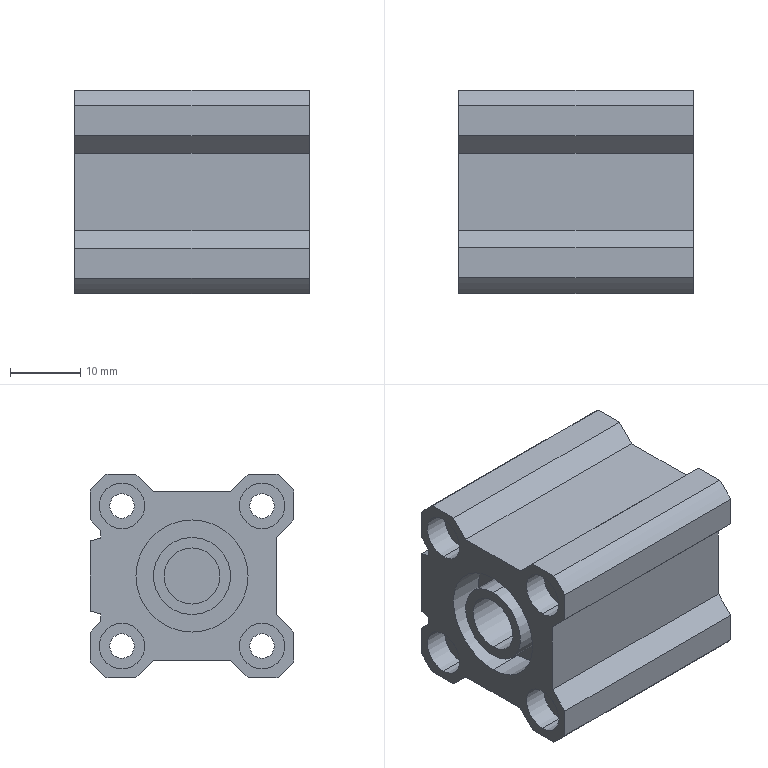Part | SolidWorks | features RefAxis 3, HoleWzd 2, LPattern 2, RevCut 2, 3DProfileFeature 1, Extrusion 1, ICE 1 | 1 solid | 87 faces | box 33.5 x 29 x 29 mm | volume 16795 mm3 | cylinder 42 | plane 41 | cone 4 | commonest cylinder face diameters 6.5 x16 3.5 x8 16 x6 4.134 x4 38 x4 8 x2